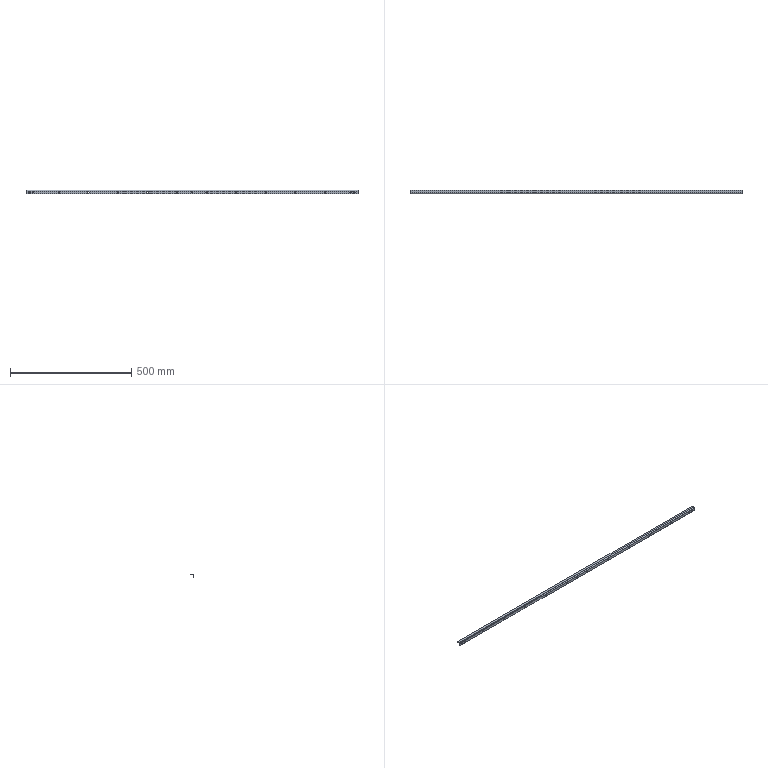Part | NX | features solid 2 | 1 solid | 40 faces | box 1368 x 13 x 15 mm | volume 66765 mm3 | cylinder 32 | plane 8 | commonest cylinder face diameters 6 x30 4 x1 8 x1
STEP:
#1=CARTESIAN_POINT('',(-726.,-675.5,1005.5));
#2=VERTEX_POINT('',#1);
#3=CARTESIAN_POINT('',(-726.,-677.5,1005.5));
#4=VERTEX_POINT('',#3);
#5=CARTESIAN_POINT('',(-726.,-2044.644,1005.5));
#6=DIRECTION('',(0.,1.,0.));
#7=VECTOR('',#6,1000.);
#8=LINE('',#5,#7);
#9=EDGE_CURVE('',#2,#4,#8,.F.);
#10=ORIENTED_EDGE('',*,*,#9,.T.);
#11=CARTESIAN_POINT('',(-726.,-677.5,999.5));
#12=VERTEX_POINT('',#11);
#13=CARTESIAN_POINT('',(-726.,-677.5,1002.5));
#14=DIRECTION('',(0.,-1.,0.));
#15=DIRECTION('',(1.,0.,0.));
#16=AXIS2_PLACEMENT_3D('',#13,#14,#15);
#17=CIRCLE('',#16,3.);
#18=EDGE_CURVE('',#4,#12,#17,.T.);
#19=ORIENTED_EDGE('',*,*,#18,.T.);
#20=CARTESIAN_POINT('',(-726.,-675.5,999.5));
#21=VERTEX_POINT('',#20);
#22=CARTESIAN_POINT('',(-726.,-2044.644,999.5));
#23=DIRECTION('',(0.,1.,0.));
#24=VECTOR('',#23,1000.);
#25=LINE('',#22,#24);
#26=EDGE_CURVE('',#12,#21,#25,.T.);
#27=ORIENTED_EDGE('',*,*,#26,.T.);
#28=CARTESIAN_POINT('',(-726.,-675.5,1002.5));
#29=DIRECTION('',(0.,1.,0.));
#30=DIRECTION('',(-1.,0.,0.));
#31=AXIS2_PLACEMENT_3D('',#28,#29,#30);
#32=CIRCLE('',#31,3.);
#33=EDGE_CURVE('',#21,#2,#32,.T.);
#34=ORIENTED_EDGE('',*,*,#33,.T.);
#35=EDGE_LOOP('',(#10,#19,#27,#34));
#36=FACE_BOUND('',#35,.T.);
#37=CARTESIAN_POINT('',(-726.,-2044.644,1002.5));
#38=DIRECTION('',(0.,1.,0.));
#39=DIRECTION('',(0.,0.,-1.));
#40=AXIS2_PLACEMENT_3D('',#37,#38,#39);
#41=CYLINDRICAL_SURFACE('',#40,3.);
#42=ADVANCED_FACE('',(#36),#41,.F.);
#43=CARTESIAN_POINT('',(-604.273,-677.5,1005.5));
#44=VERTEX_POINT('',#43);
#45=CARTESIAN_POINT('',(-604.273,-675.5,1005.5));
#46=VERTEX_POINT('',#45);
#47=CARTESIAN_POINT('',(-604.273,-2044.644,1005.5));
#48=DIRECTION('',(0.,1.,0.));
#49=VECTOR('',#48,1000.);
#50=LINE('',#47,#49);
#51=EDGE_CURVE('',#44,#46,#50,.T.);
#52=ORIENTED_EDGE('',*,*,#51,.F.);
#53=CARTESIAN_POINT('',(-604.273,-677.5,999.5));
#54=VERTEX_POINT('',#53);
#55=CARTESIAN_POINT('',(-604.273,-677.5,1002.5));
#56=DIRECTION('',(0.,-1.,0.));
#57=DIRECTION('',(1.,0.,0.));
#58=AXIS2_PLACEMENT_3D('',#55,#56,#57);
#59=CIRCLE('',#58,3.);
#60=EDGE_CURVE('',#44,#54,#59,.T.);
#61=ORIENTED_EDGE('',*,*,#60,.T.);
#62=CARTESIAN_POINT('',(-604.273,-675.5,999.5));
#63=VERTEX_POINT('',#62);
#64=CARTESIAN_POINT('',(-604.273,-2044.644,999.5));
#65=DIRECTION('',(0.,1.,0.));
#66=VECTOR('',#65,1000.);
#67=LINE('',#64,#66);
#68=EDGE_CURVE('',#63,#54,#67,.F.);
#69=ORIENTED_EDGE('',*,*,#68,.F.);
#70=CARTESIAN_POINT('',(-604.273,-675.5,1002.5));
#71=DIRECTION('',(0.,1.,0.));
#72=DIRECTION('',(-1.,0.,0.));
#73=AXIS2_PLACEMENT_3D('',#70,#71,#72);
#74=CIRCLE('',#73,3.);
#75=EDGE_CURVE('',#63,#46,#74,.T.);
#76=ORIENTED_EDGE('',*,*,#75,.T.);
#77=EDGE_LOOP('',(#52,#61,#69,#76));
#78=FACE_BOUND('',#77,.T.);
#79=CARTESIAN_POINT('',(-604.273,-2044.644,1002.5));
#80=DIRECTION('',(0.,1.,0.));
#81=DIRECTION('',(0.,0.,-1.));
#82=AXIS2_PLACEMENT_3D('',#79,#80,#81);
#83=CYLINDRICAL_SURFACE('',#82,3.);
#84=ADVANCED_FACE('',(#78),#83,.F.);
#85=CARTESIAN_POINT('',(-482.545,-675.5,1005.5));
#86=VERTEX_POINT('',#85);
#87=CARTESIAN_POINT('',(-482.545,-677.5,1005.5));
#88=VERTEX_POINT('',#87);
#89=CARTESIAN_POINT('',(-482.545,-2044.644,1005.5));
#90=DIRECTION('',(0.,1.,0.));
#91=VECTOR('',#90,1000.);
#92=LINE('',#89,#91);
#93=EDGE_CURVE('',#86,#88,#92,.F.);
#94=ORIENTED_EDGE('',*,*,#93,.T.);
#95=CARTESIAN_POINT('',(-482.545,-677.5,999.5));
#96=VERTEX_POINT('',#95);
#97=CARTESIAN_POINT('',(-482.545,-677.5,1002.5));
#98=DIRECTION('',(0.,-1.,0.));
#99=DIRECTION('',(1.,0.,0.));
#100=AXIS2_PLACEMENT_3D('',#97,#98,#99);
#101=CIRCLE('',#100,3.);
#102=EDGE_CURVE('',#88,#96,#101,.T.);
#103=ORIENTED_EDGE('',*,*,#102,.T.);
#104=CARTESIAN_POINT('',(-482.545,-675.5,999.5));
#105=VERTEX_POINT('',#104);
#106=CARTESIAN_POINT('',(-482.545,-2044.644,999.5));
#107=DIRECTION('',(0.,1.,0.));
#108=VECTOR('',#107,1000.);
#109=LINE('',#106,#108);
#110=EDGE_CURVE('',#96,#105,#109,.T.);
#111=ORIENTED_EDGE('',*,*,#110,.T.);
#112=CARTESIAN_POINT('',(-482.545,-675.5,1002.5));
#113=DIRECTION('',(0.,1.,0.));
#114=DIRECTION('',(-1.,0.,0.));
#115=AXIS2_PLACEMENT_3D('',#112,#113,#114);
#116=CIRCLE('',#115,3.);
#117=EDGE_CURVE('',#105,#86,#116,.T.);
#118=ORIENTED_EDGE('',*,*,#117,.T.);
#119=EDGE_LOOP('',(#94,#103,#111,#118));
#120=FACE_BOUND('',#119,.T.);
#121=CARTESIAN_POINT('',(-482.545,-2044.644,1002.5));
#122=DIRECTION('',(0.,1.,0.));
#123=DIRECTION('',(0.,0.,-1.));
#124=AXIS2_PLACEMENT_3D('',#121,#122,#123);
#125=CYLINDRICAL_SURFACE('',#124,3.);
#126=ADVANCED_FACE('',(#120),#125,.F.);
#127=CARTESIAN_POINT('',(-360.818,-675.5,1005.5));
#128=VERTEX_POINT('',#127);
#129=CARTESIAN_POINT('',(-360.818,-677.5,1005.5));
#130=VERTEX_POINT('',#129);
#131=CARTESIAN_POINT('',(-360.818,-2044.644,1005.5));
#132=DIRECTION('',(0.,1.,0.));
#133=VECTOR('',#132,1000.);
#134=LINE('',#131,#133);
#135=EDGE_CURVE('',#128,#130,#134,.F.);
#136=ORIENTED_EDGE('',*,*,#135,.T.);
#137=CARTESIAN_POINT('',(-360.818,-677.5,999.5));
#138=VERTEX_POINT('',#137);
#139=CARTESIAN_POINT('',(-360.818,-677.5,1002.5));
#140=DIRECTION('',(0.,-1.,0.));
#141=DIRECTION('',(1.,0.,0.));
#142=AXIS2_PLACEMENT_3D('',#139,#140,#141);
#143=CIRCLE('',#142,3.);
#144=EDGE_CURVE('',#130,#138,#143,.T.);
#145=ORIENTED_EDGE('',*,*,#144,.T.);
#146=CARTESIAN_POINT('',(-360.818,-675.5,999.5));
#147=VERTEX_POINT('',#146);
#148=CARTESIAN_POINT('',(-360.818,-2044.644,999.5));
#149=DIRECTION('',(0.,1.,0.));
#150=VECTOR('',#149,1000.);
#151=LINE('',#148,#150);
#152=EDGE_CURVE('',#138,#147,#151,.T.);
#153=ORIENTED_EDGE('',*,*,#152,.T.);
#154=CARTESIAN_POINT('',(-360.818,-675.5,1002.5));
#155=DIRECTION('',(0.,1.,0.));
#156=DIRECTION('',(-1.,0.,0.));
#157=AXIS2_PLACEMENT_3D('',#154,#155,#156);
#158=CIRCLE('',#157,3.);
#159=EDGE_CURVE('',#147,#128,#158,.T.);
#160=ORIENTED_EDGE('',*,*,#159,.T.);
#161=EDGE_LOOP('',(#136,#145,#153,#160));
#162=FACE_BOUND('',#161,.T.);
#163=CARTESIAN_POINT('',(-360.818,-2044.644,1002.5));
#164=DIRECTION('',(0.,1.,0.));
#165=DIRECTION('',(0.,0.,-1.));
#166=AXIS2_PLACEMENT_3D('',#163,#164,#165);
#167=CYLINDRICAL_SURFACE('',#166,3.);
#168=ADVANCED_FACE('',(#162),#167,.F.);
#169=CARTESIAN_POINT('',(-239.091,-677.5,1005.5));
#170=VERTEX_POINT('',#169);
#171=CARTESIAN_POINT('',(-239.091,-675.5,1005.5));
#172=VERTEX_POINT('',#171);
#173=CARTESIAN_POINT('',(-239.091,-2044.644,1005.5));
#174=DIRECTION('',(0.,1.,0.));
#175=VECTOR('',#174,1000.);
#176=LINE('',#173,#175);
#177=EDGE_CURVE('',#170,#172,#176,.T.);
#178=ORIENTED_EDGE('',*,*,#177,.F.);
#179=CARTESIAN_POINT('',(-239.091,-677.5,999.5));
#180=VERTEX_POINT('',#179);
#181=CARTESIAN_POINT('',(-239.091,-677.5,1002.5));
#182=DIRECTION('',(0.,-1.,0.));
#183=DIRECTION('',(1.,0.,0.));
#184=AXIS2_PLACEMENT_3D('',#181,#182,#183);
#185=CIRCLE('',#184,3.);
#186=EDGE_CURVE('',#170,#180,#185,.T.);
#187=ORIENTED_EDGE('',*,*,#186,.T.);
#188=CARTESIAN_POINT('',(-239.091,-675.5,999.5));
#189=VERTEX_POINT('',#188);
#190=CARTESIAN_POINT('',(-239.091,-2044.644,999.5));
#191=DIRECTION('',(0.,1.,0.));
#192=VECTOR('',#191,1000.);
#193=LINE('',#190,#192);
#194=EDGE_CURVE('',#189,#180,#193,.F.);
#195=ORIENTED_EDGE('',*,*,#194,.F.);
#196=CARTESIAN_POINT('',(-239.091,-675.5,1002.5));
#197=DIRECTION('',(0.,1.,0.));
#198=DIRECTION('',(-1.,0.,0.));
#199=AXIS2_PLACEMENT_3D('',#196,#197,#198);
#200=CIRCLE('',#199,3.);
#201=EDGE_CURVE('',#189,#172,#200,.T.);
#202=ORIENTED_EDGE('',*,*,#201,.T.);
#203=EDGE_LOOP('',(#178,#187,#195,#202));
#204=FACE_BOUND('',#203,.T.);
#205=CARTESIAN_POINT('',(-239.091,-2044.644,1002.5));
#206=DIRECTION('',(0.,1.,0.));
#207=DIRECTION('',(0.,0.,-1.));
#208=AXIS2_PLACEMENT_3D('',#205,#206,#207);
#209=CYLINDRICAL_SURFACE('',#208,3.);
#210=ADVANCED_FACE('',(#204),#209,.F.);
#211=CARTESIAN_POINT('',(-117.364,-675.5,1005.5));
#212=VERTEX_POINT('',#211);
#213=CARTESIAN_POINT('',(-117.364,-677.5,1005.5));
#214=VERTEX_POINT('',#213);
#215=CARTESIAN_POINT('',(-117.364,-2044.644,1005.5));
#216=DIRECTION('',(0.,1.,0.));
#217=VECTOR('',#216,1000.);
#218=LINE('',#215,#217);
#219=EDGE_CURVE('',#212,#214,#218,.F.);
#220=ORIENTED_EDGE('',*,*,#219,.T.);
#221=CARTESIAN_POINT('',(-117.364,-677.5,999.5));
#222=VERTEX_POINT('',#221);
#223=CARTESIAN_POINT('',(-117.364,-677.5,1002.5));
#224=DIRECTION('',(0.,-1.,0.));
#225=DIRECTION('',(1.,0.,0.));
#226=AXIS2_PLACEMENT_3D('',#223,#224,#225);
#227=CIRCLE('',#226,3.);
#228=EDGE_CURVE('',#214,#222,#227,.T.);
#229=ORIENTED_EDGE('',*,*,#228,.T.);
#230=CARTESIAN_POINT('',(-117.364,-675.5,999.5));
#231=VERTEX_POINT('',#230);
#232=CARTESIAN_POINT('',(-117.364,-2044.644,999.5));
#233=DIRECTION('',(0.,1.,0.));
#234=VECTOR('',#233,1000.);
#235=LINE('',#232,#234);
#236=EDGE_CURVE('',#222,#231,#235,.T.);
#237=ORIENTED_EDGE('',*,*,#236,.T.);
#238=CARTESIAN_POINT('',(-117.364,-675.5,1002.5));
#239=DIRECTION('',(0.,1.,0.));
#240=DIRECTION('',(-1.,0.,0.));
#241=AXIS2_PLACEMENT_3D('',#238,#239,#240);
#242=CIRCLE('',#241,3.);
#243=EDGE_CURVE('',#231,#212,#242,.T.);
#244=ORIENTED_EDGE('',*,*,#243,.T.);
#245=EDGE_LOOP('',(#220,#229,#237,#244));
#246=FACE_BOUND('',#245,.T.);
#247=CARTESIAN_POINT('',(-117.364,-2044.644,1002.5));
#248=DIRECTION('',(0.,1.,0.));
#249=DIRECTION('',(0.,0.,-1.));
#250=AXIS2_PLACEMENT_3D('',#247,#248,#249);
#251=CYLINDRICAL_SURFACE('',#250,3.);
#252=ADVANCED_FACE('',(#246),#251,.F.);
#253=CARTESIAN_POINT('',(4.364,-677.5,1005.5));
#254=VERTEX_POINT('',#253);
#255=CARTESIAN_POINT('',(4.364,-675.5,1005.5));
#256=VERTEX_POINT('',#255);
#257=CARTESIAN_POINT('',(4.364,-2044.644,1005.5));
#258=DIRECTION('',(0.,1.,0.));
#259=VECTOR('',#258,1000.);
#260=LINE('',#257,#259);
#261=EDGE_CURVE('',#254,#256,#260,.T.);
#262=ORIENTED_EDGE('',*,*,#261,.F.);
#263=CARTESIAN_POINT('',(4.364,-677.5,999.5));
#264=VERTEX_POINT('',#263);
#265=CARTESIAN_POINT('',(4.364,-677.5,1002.5));
#266=DIRECTION('',(0.,-1.,0.));
#267=DIRECTION('',(1.,0.,0.));
#268=AXIS2_PLACEMENT_3D('',#265,#266,#267);
#269=CIRCLE('',#268,3.);
#270=EDGE_CURVE('',#254,#264,#269,.T.);
#271=ORIENTED_EDGE('',*,*,#270,.T.);
#272=CARTESIAN_POINT('',(4.364,-675.5,999.5));
#273=VERTEX_POINT('',#272);
#274=CARTESIAN_POINT('',(4.364,-2044.644,999.5));
#275=DIRECTION('',(0.,1.,0.));
#276=VECTOR('',#275,1000.);
#277=LINE('',#274,#276);
#278=EDGE_CURVE('',#273,#264,#277,.F.);
#279=ORIENTED_EDGE('',*,*,#278,.F.);
#280=CARTESIAN_POINT('',(4.364,-675.5,1002.5));
#281=DIRECTION('',(0.,1.,0.));
#282=DIRECTION('',(-1.,0.,0.));
#283=AXIS2_PLACEMENT_3D('',#280,#281,#282);
#284=CIRCLE('',#283,3.);
#285=EDGE_CURVE('',#273,#256,#284,.T.);
#286=ORIENTED_EDGE('',*,*,#285,.T.);
#287=EDGE_LOOP('',(#262,#271,#279,#286));
#288=FACE_BOUND('',#287,.T.);
#289=CARTESIAN_POINT('',(4.364,-2044.644,1002.5));
#290=DIRECTION('',(0.,1.,0.));
#291=DIRECTION('',(0.,0.,-1.));
#292=AXIS2_PLACEMENT_3D('',#289,#290,#291);
#293=CYLINDRICAL_SURFACE('',#292,3.);
#294=ADVANCED_FACE('',(#288),#293,.F.);
#295=CARTESIAN_POINT('',(126.091,-675.5,1005.5));
#296=VERTEX_POINT('',#295);
#297=CARTESIAN_POINT('',(126.091,-677.5,1005.5));
#298=VERTEX_POINT('',#297);
#299=CARTESIAN_POINT('',(126.091,-2044.644,1005.5));
#300=DIRECTION('',(0.,1.,0.));
#301=VECTOR('',#300,1000.);
#302=LINE('',#299,#301);
#303=EDGE_CURVE('',#296,#298,#302,.F.);
#304=ORIENTED_EDGE('',*,*,#303,.T.);
#305=CARTESIAN_POINT('',(126.091,-677.5,999.5));
#306=VERTEX_POINT('',#305);
#307=CARTESIAN_POINT('',(126.091,-677.5,1002.5));
#308=DIRECTION('',(0.,-1.,0.));
#309=DIRECTION('',(1.,0.,0.));
#310=AXIS2_PLACEMENT_3D('',#307,#308,#309);
#311=CIRCLE('',#310,3.);
#312=EDGE_CURVE('',#298,#306,#311,.T.);
#313=ORIENTED_EDGE('',*,*,#312,.T.);
#314=CARTESIAN_POINT('',(126.091,-675.5,999.5));
#315=VERTEX_POINT('',#314);
#316=CARTESIAN_POINT('',(126.091,-2044.644,999.5));
#317=DIRECTION('',(0.,1.,0.));
#318=VECTOR('',#317,1000.);
#319=LINE('',#316,#318);
#320=EDGE_CURVE('',#306,#315,#319,.T.);
#321=ORIENTED_EDGE('',*,*,#320,.T.);
#322=CARTESIAN_POINT('',(126.091,-675.5,1002.5));
#323=DIRECTION('',(0.,1.,0.));
#324=DIRECTION('',(-1.,0.,0.));
#325=AXIS2_PLACEMENT_3D('',#322,#323,#324);
#326=CIRCLE('',#325,3.);
#327=EDGE_CURVE('',#315,#296,#326,.T.);
#328=ORIENTED_EDGE('',*,*,#327,.T.);
#329=EDGE_LOOP('',(#304,#313,#321,#328));
#330=FACE_BOUND('',#329,.T.);
#331=CARTESIAN_POINT('',(126.091,-2044.644,1002.5));
#332=DIRECTION('',(0.,1.,0.));
#333=DIRECTION('',(0.,0.,-1.));
#334=AXIS2_PLACEMENT_3D('',#331,#332,#333);
#335=CYLINDRICAL_SURFACE('',#334,3.);
#336=ADVANCED_FACE('',(#330),#335,.F.);
#337=CARTESIAN_POINT('',(247.818,-675.5,1005.5));
#338=VERTEX_POINT('',#337);
#339=CARTESIAN_POINT('',(247.818,-677.5,1005.5));
#340=VERTEX_POINT('',#339);
#341=CARTESIAN_POINT('',(247.818,-2044.644,1005.5));
#342=DIRECTION('',(0.,1.,0.));
#343=VECTOR('',#342,1000.);
#344=LINE('',#341,#343);
#345=EDGE_CURVE('',#338,#340,#344,.F.);
#346=ORIENTED_EDGE('',*,*,#345,.T.);
#347=CARTESIAN_POINT('',(247.818,-677.5,999.5));
#348=VERTEX_POINT('',#347);
#349=CARTESIAN_POINT('',(247.818,-677.5,1002.5));
#350=DIRECTION('',(0.,-1.,0.));
#351=DIRECTION('',(1.,0.,0.));
#352=AXIS2_PLACEMENT_3D('',#349,#350,#351);
#353=CIRCLE('',#352,3.);
#354=EDGE_CURVE('',#340,#348,#353,.T.);
#355=ORIENTED_EDGE('',*,*,#354,.T.);
#356=CARTESIAN_POINT('',(247.818,-675.5,999.5));
#357=VERTEX_POINT('',#356);
#358=CARTESIAN_POINT('',(247.818,-2044.644,999.5));
#359=DIRECTION('',(0.,1.,0.));
#360=VECTOR('',#359,1000.);
#361=LINE('',#358,#360);
#362=EDGE_CURVE('',#348,#357,#361,.T.);
#363=ORIENTED_EDGE('',*,*,#362,.T.);
#364=CARTESIAN_POINT('',(247.818,-675.5,1002.5));
#365=DIRECTION('',(0.,1.,0.));
#366=DIRECTION('',(-1.,0.,0.));
#367=AXIS2_PLACEMENT_3D('',#364,#365,#366);
#368=CIRCLE('',#367,3.);
#369=EDGE_CURVE('',#357,#338,#368,.T.);
#370=ORIENTED_EDGE('',*,*,#369,.T.);
#371=EDGE_LOOP('',(#346,#355,#363,#370));
#372=FACE_BOUND('',#371,.T.);
#373=CARTESIAN_POINT('',(247.818,-2044.644,1002.5));
#374=DIRECTION('',(0.,1.,0.));
#375=DIRECTION('',(0.,0.,-1.));
#376=AXIS2_PLACEMENT_3D('',#373,#374,#375);
#377=CYLINDRICAL_SURFACE('',#376,3.);
#378=ADVANCED_FACE('',(#372),#377,.F.);
#379=CARTESIAN_POINT('',(369.545,-677.5,1005.5));
#380=VERTEX_POINT('',#379);
#381=CARTESIAN_POINT('',(369.545,-675.5,1005.5));
#382=VERTEX_POINT('',#381);
#383=CARTESIAN_POINT('',(369.545,-2044.644,1005.5));
#384=DIRECTION('',(0.,1.,0.));
#385=VECTOR('',#384,1000.);
#386=LINE('',#383,#385);
#387=EDGE_CURVE('',#380,#382,#386,.T.);
#388=ORIENTED_EDGE('',*,*,#387,.F.);
#389=CARTESIAN_POINT('',(369.545,-677.5,999.5));
#390=VERTEX_POINT('',#389);
#391=CARTESIAN_POINT('',(369.545,-677.5,1002.5));
#392=DIRECTION('',(0.,-1.,0.));
#393=DIRECTION('',(1.,0.,0.));
#394=AXIS2_PLACEMENT_3D('',#391,#392,#393);
#395=CIRCLE('',#394,3.);
#396=EDGE_CURVE('',#380,#390,#395,.T.);
#397=ORIENTED_EDGE('',*,*,#396,.T.);
#398=CARTESIAN_POINT('',(369.545,-675.5,999.5));
#399=VERTEX_POINT('',#398);
#400=CARTESIAN_POINT('',(369.545,-2044.644,999.5));
#401=DIRECTION('',(0.,1.,0.));
#402=VECTOR('',#401,1000.);
#403=LINE('',#400,#402);
#404=EDGE_CURVE('',#399,#390,#403,.F.);
#405=ORIENTED_EDGE('',*,*,#404,.F.);
#406=CARTESIAN_POINT('',(369.545,-675.5,1002.5));
#407=DIRECTION('',(0.,1.,0.));
#408=DIRECTION('',(-1.,0.,0.));
#409=AXIS2_PLACEMENT_3D('',#406,#407,#408);
#410=CIRCLE('',#409,3.);
#411=EDGE_CURVE('',#399,#382,#410,.T.);
#412=ORIENTED_EDGE('',*,*,#411,.T.);
#413=EDGE_LOOP('',(#388,#397,#405,#412));
#414=FACE_BOUND('',#413,.T.);
#415=CARTESIAN_POINT('',(369.545,-2044.644,1002.5));
#416=DIRECTION('',(0.,1.,0.));
#417=DIRECTION('',(0.,0.,-1.));
#418=AXIS2_PLACEMENT_3D('',#415,#416,#417);
#419=CYLINDRICAL_SURFACE('',#418,3.);
#420=ADVANCED_FACE('',(#414),#419,.F.);
#421=CARTESIAN_POINT('',(491.273,-675.5,1005.5));
#422=VERTEX_POINT('',#421);
#423=CARTESIAN_POINT('',(491.273,-677.5,1005.5));
#424=VERTEX_POINT('',#423);
#425=CARTESIAN_POINT('',(491.273,-2044.644,1005.5));
#426=DIRECTION('',(0.,1.,0.));
#427=VECTOR('',#426,1000.);
#428=LINE('',#425,#427);
#429=EDGE_CURVE('',#422,#424,#428,.F.);
#430=ORIENTED_EDGE('',*,*,#429,.T.);
#431=CARTESIAN_POINT('',(491.273,-677.5,999.5));
#432=VERTEX_POINT('',#431);
#433=CARTESIAN_POINT('',(491.273,-677.5,1002.5));
#434=DIRECTION('',(0.,-1.,0.));
#435=DIRECTION('',(1.,0.,0.));
#436=AXIS2_PLACEMENT_3D('',#433,#434,#435);
#437=CIRCLE('',#436,3.);
#438=EDGE_CURVE('',#424,#432,#437,.T.);
#439=ORIENTED_EDGE('',*,*,#438,.T.);
#440=CARTESIAN_POINT('',(491.273,-675.5,999.5));
#441=VERTEX_POINT('',#440);
#442=CARTESIAN_POINT('',(491.273,-2044.644,999.5));
#443=DIRECTION('',(0.,1.,0.));
#444=VECTOR('',#443,1000.);
#445=LINE('',#442,#444);
#446=EDGE_CURVE('',#432,#441,#445,.T.);
#447=ORIENTED_EDGE('',*,*,#446,.T.);
#448=CARTESIAN_POINT('',(491.273,-675.5,1002.5));
#449=DIRECTION('',(0.,1.,0.));
#450=DIRECTION('',(-1.,0.,0.));
#451=AXIS2_PLACEMENT_3D('',#448,#449,#450);
#452=CIRCLE('',#451,3.);
#453=EDGE_CURVE('',#441,#422,#452,.T.);
#454=ORIENTED_EDGE('',*,*,#453,.T.);
#455=EDGE_LOOP('',(#430,#439,#447,#454));
#456=FACE_BOUND('',#455,.T.);
#457=CARTESIAN_POINT('',(491.273,-2044.644,1002.5));
#458=DIRECTION('',(0.,1.,0.));
#459=DIRECTION('',(0.,0.,-1.));
#460=AXIS2_PLACEMENT_3D('',#457,#458,#459);
#461=CYLINDRICAL_SURFACE('',#460,3.);
#462=ADVANCED_FACE('',(#456),#461,.F.);
#463=CARTESIAN_POINT('',(613.,-675.5,1005.5));
#464=VERTEX_POINT('',#463);
#465=CARTESIAN_POINT('',(613.,-677.5,1005.5));
#466=VERTEX_POINT('',#465);
#467=CARTESIAN_POINT('',(613.,-2044.644,1005.5));
#468=DIRECTION('',(0.,1.,0.));
#469=VECTOR('',#468,1000.);
#470=LINE('',#467,#469);
#471=EDGE_CURVE('',#464,#466,#470,.F.);
#472=ORIENTED_EDGE('',*,*,#471,.T.);
#473=CARTESIAN_POINT('',(613.,-677.5,999.5));
#474=VERTEX_POINT('',#473);
#475=CARTESIAN_POINT('',(613.,-677.5,1002.5));
#476=DIRECTION('',(0.,-1.,0.));
#477=DIRECTION('',(1.,0.,0.));
#478=AXIS2_PLACEMENT_3D('',#475,#476,#477);
#479=CIRCLE('',#478,3.);
#480=EDGE_CURVE('',#466,#474,#479,.T.);
#481=ORIENTED_EDGE('',*,*,#480,.T.);
#482=CARTESIAN_POINT('',(613.,-675.5,999.5));
#483=VERTEX_POINT('',#482);
#484=CARTESIAN_POINT('',(613.,-2044.644,999.5));
#485=DIRECTION('',(0.,1.,0.));
#486=VECTOR('',#485,1000.);
#487=LINE('',#484,#486);
#488=EDGE_CURVE('',#474,#483,#487,.T.);
#489=ORIENTED_EDGE('',*,*,#488,.T.);
#490=CARTESIAN_POINT('',(613.,-675.5,1002.5));
#491=DIRECTION('',(0.,1.,0.));
#492=DIRECTION('',(-1.,0.,0.));
#493=AXIS2_PLACEMENT_3D('',#490,#491,#492);
#494=CIRCLE('',#493,3.);
#495=EDGE_CURVE('',#483,#464,#494,.T.);
#496=ORIENTED_EDGE('',*,*,#495,.T.);
#497=EDGE_LOOP('',(#472,#481,#489,#496));
#498=FACE_BOUND('',#497,.T.);
#499=CARTESIAN_POINT('',(613.,-2044.644,1002.5));
#500=DIRECTION('',(0.,1.,0.));
#501=DIRECTION('',(0.,0.,-1.));
#502=AXIS2_PLACEMENT_3D('',#499,#500,#501);
#503=CYLINDRICAL_SURFACE('',#502,3.);
#504=ADVANCED_FACE('',(#498),#503,.F.);
#505=CARTESIAN_POINT('',(-740.,-664.5,1010.));
#506=VERTEX_POINT('',#505);
#507=CARTESIAN_POINT('',(-740.,-673.5,1010.));
#508=VERTEX_POINT('',#507);
#509=CARTESIAN_POINT('',(-740.,-677.5,1010.));
#510=DIRECTION('',(0.,-1.,0.));
#511=VECTOR('',#510,1000.);
#512=LINE('',#509,#511);
#513=EDGE_CURVE('',#506,#508,#512,.T.);
#514=ORIENTED_EDGE('',*,*,#513,.T.);
#515=CARTESIAN_POINT('',(-740.,-675.5,1008.));
#516=VERTEX_POINT('',#515);
#517=CARTESIAN_POINT('',(-740.,-673.5,1008.));
#518=DIRECTION('',(1.,0.,0.));
#519=DIRECTION('',(0.,1.,0.));
#520=AXIS2_PLACEMENT_3D('',#517,#518,#519);
#521=CIRCLE('',#520,2.);
#522=EDGE_CURVE('',#508,#516,#521,.T.);
#523=ORIENTED_EDGE('',*,*,#522,.T.);
#524=CARTESIAN_POINT('',(-740.,-675.5,997.));
#525=VERTEX_POINT('',#524);
#526=CARTESIAN_POINT('',(-740.,-675.5,1012.));
#527=DIRECTION('',(0.,0.,-1.));
#528=VECTOR('',#527,1000.);
#529=LINE('',#526,#528);
#530=EDGE_CURVE('',#516,#525,#529,.T.);
#531=ORIENTED_EDGE('',*,*,#530,.T.);
#532=CARTESIAN_POINT('',(-740.,-677.5,997.));
#533=VERTEX_POINT('',#532);
#534=CARTESIAN_POINT('',(-740.,-677.5,997.));
#535=DIRECTION('',(0.,1.,0.));
#536=VECTOR('',#535,1000.);
#537=LINE('',#534,#536);
#538=EDGE_CURVE('',#533,#525,#537,.T.);
#539=ORIENTED_EDGE('',*,*,#538,.F.);
#540=CARTESIAN_POINT('',(-740.,-677.5,1008.));
#541=VERTEX_POINT('',#540);
#542=CARTESIAN_POINT('',(-740.,-677.5,1012.));
#543=DIRECTION('',(0.,0.,-1.));
#544=VECTOR('',#543,1000.);
#545=LINE('',#542,#544);
#546=EDGE_CURVE('',#541,#533,#545,.T.);
#547=ORIENTED_EDGE('',*,*,#546,.F.);
#548=CARTESIAN_POINT('',(-740.,-673.5,1012.));
#549=VERTEX_POINT('',#548);
#550=CARTESIAN_POINT('',(-740.,-673.5,1008.));
#551=DIRECTION('',(1.,0.,0.));
#552=DIRECTION('',(0.,-1.,0.));
#553=AXIS2_PLACEMENT_3D('',#550,#551,#552);
#554=CIRCLE('',#553,4.);
#555=EDGE_CURVE('',#549,#541,#554,.T.);
#556=ORIENTED_EDGE('',*,*,#555,.F.);
#557=CARTESIAN_POINT('',(-740.,-664.5,1012.));
#558=VERTEX_POINT('',#557);
#559=CARTESIAN_POINT('',(-740.,-677.5,1012.));
#560=DIRECTION('',(0.,-1.,0.));
#561=VECTOR('',#560,1000.);
#562=LINE('',#559,#561);
#563=EDGE_CURVE('',#558,#549,#562,.T.);
#564=ORIENTED_EDGE('',*,*,#563,.F.);
#565=CARTESIAN_POINT('',(-740.,-664.5,1010.));
#566=DIRECTION('',(0.,0.,1.));
#567=VECTOR('',#566,1000.);
#568=LINE('',#565,#567);
#569=EDGE_CURVE('',#506,#558,#568,.T.);
#570=ORIENTED_EDGE('',*,*,#569,.F.);
#571=EDGE_LOOP('',(#514,#523,#531,#539,#547,#556,#564,#570));
#572=FACE_BOUND('',#571,.T.);
#573=CARTESIAN_POINT('',(-740.,-677.5,1009.5));
#574=DIRECTION('',(-1.,0.,0.));
#575=DIRECTION('',(0.,1.,0.));
#576=AXIS2_PLACEMENT_3D('',#573,#574,#575);
#577=PLANE('',#576);
#578=ADVANCED_FACE('',(#572),#577,.T.);
#579=CARTESIAN_POINT('',(628.,-664.5,1012.));
#580=VERTEX_POINT('',#579);
#581=CARTESIAN_POINT('',(628.,-673.5,1012.));
#582=VERTEX_POINT('',#581);
#583=CARTESIAN_POINT('',(628.,-677.5,1012.));
#584=DIRECTION('',(0.,-1.,0.));
#585=VECTOR('',#584,1000.);
#586=LINE('',#583,#585);
#587=EDGE_CURVE('',#580,#582,#586,.T.);
#588=ORIENTED_EDGE('',*,*,#587,.F.);
#589=CARTESIAN_POINT('',(-741.,-664.5,1012.));
#590=DIRECTION('',(1.,0.,0.));
#591=VECTOR('',#590,1000.);
#592=LINE('',#589,#591);
#593=EDGE_CURVE('',#558,#580,#592,.T.);
#594=ORIENTED_EDGE('',*,*,#593,.F.);
#595=ORIENTED_EDGE('',*,*,#563,.T.);
#596=CARTESIAN_POINT('',(-741.,-673.5,1012.));
#597=DIRECTION('',(1.,0.,0.));
#598=VECTOR('',#597,1000.);
#599=LINE('',#596,#598);
#600=EDGE_CURVE('',#549,#582,#599,.T.);
#601=ORIENTED_EDGE('',*,*,#600,.T.);
#602=EDGE_LOOP('',(#588,#594,#595,#601));
#603=FACE_BOUND('',#602,.T.);
#604=CARTESIAN_POINT('',(-741.,-677.5,1012.));
#605=DIRECTION('',(0.,0.,1.));
#606=DIRECTION('',(1.,0.,0.));
#607=AXIS2_PLACEMENT_3D('',#604,#605,#606);
#608=PLANE('',#607);
#609=ADVANCED_FACE('',(#603),#608,.T.);
#610=CARTESIAN_POINT('',(628.,-664.5,1010.));
#611=VERTEX_POINT('',#610);
#612=CARTESIAN_POINT('',(628.,-673.5,1010.));
#613=VERTEX_POINT('',#612);
#614=CARTESIAN_POINT('',(628.,-677.5,1010.));
#615=DIRECTION('',(0.,-1.,0.));
#616=VECTOR('',#615,1000.);
#617=LINE('',#614,#616);
#618=EDGE_CURVE('',#611,#613,#617,.T.);
#619=ORIENTED_EDGE('',*,*,#618,.T.);
#620=CARTESIAN_POINT('',(-741.,-673.5,1010.));
#621=DIRECTION('',(1.,0.,0.));
#622=VECTOR('',#621,1000.);
#623=LINE('',#620,#622);
#624=EDGE_CURVE('',#508,#613,#623,.T.);
#625=ORIENTED_EDGE('',*,*,#624,.F.);
#626=ORIENTED_EDGE('',*,*,#513,.F.);
#627=CARTESIAN_POINT('',(-741.,-664.5,1010.));
#628=DIRECTION('',(1.,0.,0.));
#629=VECTOR('',#628,1000.);
#630=LINE('',#627,#629);
#631=EDGE_CURVE('',#506,#611,#630,.T.);
#632=ORIENTED_EDGE('',*,*,#631,.T.);
#633=EDGE_LOOP('',(#619,#625,#626,#632));
#634=FACE_BOUND('',#633,.T.);
#635=CARTESIAN_POINT('',(-741.,-677.5,1010.));
#636=DIRECTION('',(0.,0.,1.));
#637=DIRECTION('',(1.,0.,0.));
#638=AXIS2_PLACEMENT_3D('',#635,#636,#637);
#639=PLANE('',#638);
#640=ADVANCED_FACE('',(#634),#639,.F.);
#641=CARTESIAN_POINT('',(628.,-664.5,1010.));
#642=DIRECTION('',(0.,0.,1.));
#643=VECTOR('',#642,1000.);
#644=LINE('',#641,#643);
#645=EDGE_CURVE('',#611,#580,#644,.T.);
#646=ORIENTED_EDGE('',*,*,#645,.F.);
#647=ORIENTED_EDGE('',*,*,#631,.F.);
#648=ORIENTED_EDGE('',*,*,#569,.T.);
#649=ORIENTED_EDGE('',*,*,#593,.T.);
#650=EDGE_LOOP('',(#646,#647,#648,#649));
#651=FACE_BOUND('',#650,.T.);
#652=CARTESIAN_POINT('',(-741.,-664.5,1010.));
#653=DIRECTION('',(0.,1.,0.));
#654=DIRECTION('',(0.,0.,-1.));
#655=AXIS2_PLACEMENT_3D('',#652,#653,#654);
#656=PLANE('',#655);
#657=ADVANCED_FACE('',(#651),#656,.T.);
#658=ORIENTED_EDGE('',*,*,#522,.F.);
#659=ORIENTED_EDGE('',*,*,#624,.T.);
#660=CARTESIAN_POINT('',(628.,-675.5,1008.));
#661=VERTEX_POINT('',#660);
#662=CARTESIAN_POINT('',(628.,-673.5,1008.));
#663=DIRECTION('',(1.,0.,0.));
#664=DIRECTION('',(0.,1.,0.));
#665=AXIS2_PLACEMENT_3D('',#662,#663,#664);
#666=CIRCLE('',#665,2.);
#667=EDGE_CURVE('',#613,#661,#666,.T.);
#668=ORIENTED_EDGE('',*,*,#667,.T.);
#669=CARTESIAN_POINT('',(-741.,-675.5,1008.));
#670=DIRECTION('',(1.,0.,0.));
#671=VECTOR('',#670,1000.);
#672=LINE('',#669,#671);
#673=EDGE_CURVE('',#516,#661,#672,.T.);
#674=ORIENTED_EDGE('',*,*,#673,.F.);
#675=EDGE_LOOP('',(#658,#659,#668,#674));
#676=FACE_BOUND('',#675,.T.);
#677=CARTESIAN_POINT('',(-741.,-673.5,1008.));
#678=DIRECTION('',(1.,0.,0.));
#679=DIRECTION('',(0.,-1.,0.));
#680=AXIS2_PLACEMENT_3D('',#677,#678,#679);
#681=CYLINDRICAL_SURFACE('',#680,2.);
#682=ADVANCED_FACE('',(#676),#681,.F.);
#683=ORIENTED_EDGE('',*,*,#555,.T.);
#684=CARTESIAN_POINT('',(628.,-677.5,1008.));
#685=VERTEX_POINT('',#684);
#686=CARTESIAN_POINT('',(-741.,-677.5,1008.));
#687=DIRECTION('',(1.,0.,0.));
#688=VECTOR('',#687,1000.);
#689=LINE('',#686,#688);
#690=EDGE_CURVE('',#541,#685,#689,.T.);
#691=ORIENTED_EDGE('',*,*,#690,.T.);
#692=CARTESIAN_POINT('',(628.,-673.5,1008.));
#693=DIRECTION('',(1.,0.,0.));
#694=DIRECTION('',(0.,-1.,0.));
#695=AXIS2_PLACEMENT_3D('',#692,#693,#694);
#696=CIRCLE('',#695,4.);
#697=EDGE_CURVE('',#582,#685,#696,.T.);
#698=ORIENTED_EDGE('',*,*,#697,.F.);
#699=ORIENTED_EDGE('',*,*,#600,.F.);
#700=EDGE_LOOP('',(#683,#691,#698,#699));
#701=FACE_BOUND('',#700,.T.);
#702=CARTESIAN_POINT('',(-741.,-673.5,1008.));
#703=DIRECTION('',(1.,0.,0.));
#704=DIRECTION('',(0.,-1.,0.));
#705=AXIS2_PLACEMENT_3D('',#702,#703,#704);
#706=CYLINDRICAL_SURFACE('',#705,4.);
#707=ADVANCED_FACE('',(#701),#706,.T.);
#708=CARTESIAN_POINT('',(-711.,-675.5,1007.));
#709=VERTEX_POINT('',#708);
#710=CARTESIAN_POINT('',(-711.,-677.5,1007.));
#711=VERTEX_POINT('',#710);
#712=CARTESIAN_POINT('',(-711.,-2012.147,1007.));
#713=DIRECTION('',(0.,1.,0.));
#714=VECTOR('',#713,1000.);
#715=LINE('',#712,#714);
#716=EDGE_CURVE('',#709,#711,#715,.F.);
#717=ORIENTED_EDGE('',*,*,#716,.T.);
#718=CARTESIAN_POINT('',(-711.,-677.5,1001.));
#719=VERTEX_POINT('',#718);
#720=CARTESIAN_POINT('',(-711.,-677.5,1004.));
#721=DIRECTION('',(0.,-1.,0.));
#722=DIRECTION('',(1.,0.,0.));
#723=AXIS2_PLACEMENT_3D('',#720,#721,#722);
#724=CIRCLE('',#723,3.);
#725=EDGE_CURVE('',#711,#719,#724,.T.);
#726=ORIENTED_EDGE('',*,*,#725,.T.);
#727=CARTESIAN_POINT('',(-711.,-675.5,1001.));
#728=VERTEX_POINT('',#727);
#729=CARTESIAN_POINT('',(-711.,-2012.147,1001.));
#730=DIRECTION('',(0.,1.,0.));
#731=VECTOR('',#730,1000.);
#732=LINE('',#729,#731);
#733=EDGE_CURVE('',#719,#728,#732,.T.);
#734=ORIENTED_EDGE('',*,*,#733,.T.);
#735=CARTESIAN_POINT('',(-711.,-675.5,1004.));
#736=DIRECTION('',(0.,1.,0.));
#737=DIRECTION('',(1.,0.,0.));
#738=AXIS2_PLACEMENT_3D('',#735,#736,#737);
#739=CIRCLE('',#738,3.);
#740=EDGE_CURVE('',#728,#709,#739,.T.);
#741=ORIENTED_EDGE('',*,*,#740,.T.);
#742=EDGE_LOOP('',(#717,#726,#734,#741));
#743=FACE_BOUND('',#742,.T.);
#744=CARTESIAN_POINT('',(-711.,-2012.147,1004.));
#745=DIRECTION('',(0.,1.,0.));
#746=DIRECTION('',(0.,0.,-1.));
#747=AXIS2_PLACEMENT_3D('',#744,#745,#746);
#748=CYLINDRICAL_SURFACE('',#747,3.);
#749=ADVANCED_FACE('',(#743),#748,.F.);
#750=CARTESIAN_POINT('',(-56.5,-677.5,1007.));
#751=VERTEX_POINT('',#750);
#752=CARTESIAN_POINT('',(-56.5,-675.5,1007.));
#753=VERTEX_POINT('',#752);
#754=CARTESIAN_POINT('',(-56.5,-2012.147,1007.));
#755=DIRECTION('',(0.,1.,0.));
#756=VECTOR('',#755,1000.);
#757=LINE('',#754,#756);
#758=EDGE_CURVE('',#751,#753,#757,.T.);
#759=ORIENTED_EDGE('',*,*,#758,.F.);
#760=CARTESIAN_POINT('',(-56.5,-677.5,1001.));
#761=VERTEX_POINT('',#760);
#762=CARTESIAN_POINT('',(-56.5,-677.5,1004.));
#763=DIRECTION('',(0.,-1.,0.));
#764=DIRECTION('',(1.,0.,0.));
#765=AXIS2_PLACEMENT_3D('',#762,#763,#764);
#766=CIRCLE('',#765,3.);
#767=EDGE_CURVE('',#751,#761,#766,.T.);
#768=ORIENTED_EDGE('',*,*,#767,.T.);
#769=CARTESIAN_POINT('',(-56.5,-675.5,1001.));
#770=VERTEX_POINT('',#769);
#771=CARTESIAN_POINT('',(-56.5,-2012.147,1001.));
#772=DIRECTION('',(0.,1.,0.));
#773=VECTOR('',#772,1000.);
#774=LINE('',#771,#773);
#775=EDGE_CURVE('',#770,#761,#774,.F.);
#776=ORIENTED_EDGE('',*,*,#775,.F.);
#777=CARTESIAN_POINT('',(-56.5,-675.5,1004.));
#778=DIRECTION('',(0.,1.,0.));
#779=DIRECTION('',(1.,0.,0.));
#780=AXIS2_PLACEMENT_3D('',#777,#778,#779);
#781=CIRCLE('',#780,3.);
#782=EDGE_CURVE('',#770,#753,#781,.T.);
#783=ORIENTED_EDGE('',*,*,#782,.T.);
#784=EDGE_LOOP('',(#759,#768,#776,#783));
#785=FACE_BOUND('',#784,.T.);
#786=CARTESIAN_POINT('',(-56.5,-2012.147,1004.));
#787=DIRECTION('',(0.,1.,0.));
#788=DIRECTION('',(0.,0.,-1.));
#789=AXIS2_PLACEMENT_3D('',#786,#787,#788);
#790=CYLINDRICAL_SURFACE('',#789,3.);
#791=ADVANCED_FACE('',(#785),#790,.F.);
#792=CARTESIAN_POINT('',(598.,-677.5,1007.));
#793=VERTEX_POINT('',#792);
#794=CARTESIAN_POINT('',(598.,-675.5,1007.));
#795=VERTEX_POINT('',#794);
#796=CARTESIAN_POINT('',(598.,-2012.147,1007.));
#797=DIRECTION('',(0.,1.,0.));
#798=VECTOR('',#797,1000.);
#799=LINE('',#796,#798);
#800=EDGE_CURVE('',#793,#795,#799,.T.);
#801=ORIENTED_EDGE('',*,*,#800,.F.);
#802=CARTESIAN_POINT('',(598.,-677.5,1001.));
#803=VERTEX_POINT('',#802);
#804=CARTESIAN_POINT('',(598.,-677.5,1004.));
#805=DIRECTION('',(0.,-1.,0.));
#806=DIRECTION('',(1.,0.,0.));
#807=AXIS2_PLACEMENT_3D('',#804,#805,#806);
#808=CIRCLE('',#807,3.);
#809=EDGE_CURVE('',#793,#803,#808,.T.);
#810=ORIENTED_EDGE('',*,*,#809,.T.);
#811=CARTESIAN_POINT('',(598.,-675.5,1001.));
#812=VERTEX_POINT('',#811);
#813=CARTESIAN_POINT('',(598.,-2012.147,1001.));
#814=DIRECTION('',(0.,1.,0.));
#815=VECTOR('',#814,1000.);
#816=LINE('',#813,#815);
#817=EDGE_CURVE('',#812,#803,#816,.F.);
#818=ORIENTED_EDGE('',*,*,#817,.F.);
#819=CARTESIAN_POINT('',(598.,-675.5,1004.));
#820=DIRECTION('',(0.,1.,0.));
#821=DIRECTION('',(1.,0.,0.));
#822=AXIS2_PLACEMENT_3D('',#819,#820,#821);
#823=CIRCLE('',#822,3.);
#824=EDGE_CURVE('',#812,#795,#823,.T.);
#825=ORIENTED_EDGE('',*,*,#824,.T.);
#826=EDGE_LOOP('',(#801,#810,#818,#825));
#827=FACE_BOUND('',#826,.T.);
#828=CARTESIAN_POINT('',(598.,-2012.147,1004.));
#829=DIRECTION('',(0.,1.,0.));
#830=DIRECTION('',(0.,0.,-1.));
#831=AXIS2_PLACEMENT_3D('',#828,#829,#830);
#832=CYLINDRICAL_SURFACE('',#831,3.);
#833=ADVANCED_FACE('',(#827),#832,.F.);
#834=ORIENTED_EDGE('',*,*,#824,.F.);
#835=CARTESIAN_POINT('',(598.,-675.5,1004.));
#836=DIRECTION('',(0.,1.,0.));
#837=DIRECTION('',(1.,0.,0.));
#838=AXIS2_PLACEMENT_3D('',#835,#836,#837);
#839=CIRCLE('',#838,3.);
#840=EDGE_CURVE('',#795,#812,#839,.T.);
#841=ORIENTED_EDGE('',*,*,#840,.F.);
#842=EDGE_LOOP('',(#834,#841));
#843=FACE_BOUND('',#842,.T.);
#844=ORIENTED_EDGE('',*,*,#782,.F.);
#845=CARTESIAN_POINT('',(-56.5,-675.5,1004.));
#846=DIRECTION('',(0.,1.,0.));
#847=DIRECTION('',(1.,0.,0.));
#848=AXIS2_PLACEMENT_3D('',#845,#846,#847);
#849=CIRCLE('',#848,3.);
#850=EDGE_CURVE('',#753,#770,#849,.T.);
#851=ORIENTED_EDGE('',*,*,#850,.F.);
#852=EDGE_LOOP('',(#844,#851));
#853=FACE_BOUND('',#852,.T.);
#854=ORIENTED_EDGE('',*,*,#740,.F.);
#855=CARTESIAN_POINT('',(-711.,-675.5,1004.));
#856=DIRECTION('',(0.,1.,0.));
#857=DIRECTION('',(1.,0.,0.));
#858=AXIS2_PLACEMENT_3D('',#855,#856,#857);
#859=CIRCLE('',#858,3.);
#860=EDGE_CURVE('',#709,#728,#859,.T.);
#861=ORIENTED_EDGE('',*,*,#860,.F.);
#862=EDGE_LOOP('',(#854,#861));
#863=FACE_BOUND('',#862,.T.);
#864=ORIENTED_EDGE('',*,*,#495,.F.);
#865=CARTESIAN_POINT('',(613.,-675.5,1002.5));
#866=DIRECTION('',(0.,1.,0.));
#867=DIRECTION('',(-1.,0.,0.));
#868=AXIS2_PLACEMENT_3D('',#865,#866,#867);
#869=CIRCLE('',#868,3.);
#870=EDGE_CURVE('',#464,#483,#869,.T.);
#871=ORIENTED_EDGE('',*,*,#870,.F.);
#872=EDGE_LOOP('',(#864,#871));
#873=FACE_BOUND('',#872,.T.);
#874=ORIENTED_EDGE('',*,*,#453,.F.);
#875=CARTESIAN_POINT('',(491.273,-675.5,1002.5));
#876=DIRECTION('',(0.,1.,0.));
#877=DIRECTION('',(-1.,0.,0.));
#878=AXIS2_PLACEMENT_3D('',#875,#876,#877);
#879=CIRCLE('',#878,3.);
#880=EDGE_CURVE('',#422,#441,#879,.T.);
#881=ORIENTED_EDGE('',*,*,#880,.F.);
#882=EDGE_LOOP('',(#874,#881));
#883=FACE_BOUND('',#882,.T.);
#884=ORIENTED_EDGE('',*,*,#411,.F.);
#885=CARTESIAN_POINT('',(369.545,-675.5,1002.5));
#886=DIRECTION('',(0.,1.,0.));
#887=DIRECTION('',(-1.,0.,0.));
#888=AXIS2_PLACEMENT_3D('',#885,#886,#887);
#889=CIRCLE('',#888,3.);
#890=EDGE_CURVE('',#382,#399,#889,.T.);
#891=ORIENTED_EDGE('',*,*,#890,.F.);
#892=EDGE_LOOP('',(#884,#891));
#893=FACE_BOUND('',#892,.T.);
#894=ORIENTED_EDGE('',*,*,#369,.F.);
#895=CARTESIAN_POINT('',(247.818,-675.5,1002.5));
#896=DIRECTION('',(0.,1.,0.));
#897=DIRECTION('',(-1.,0.,0.));
#898=AXIS2_PLACEMENT_3D('',#895,#896,#897);
#899=CIRCLE('',#898,3.);
#900=EDGE_CURVE('',#338,#357,#899,.T.);
#901=ORIENTED_EDGE('',*,*,#900,.F.);
#902=EDGE_LOOP('',(#894,#901));
#903=FACE_BOUND('',#902,.T.);
#904=ORIENTED_EDGE('',*,*,#327,.F.);
#905=CARTESIAN_POINT('',(126.091,-675.5,1002.5));
#906=DIRECTION('',(0.,1.,0.));
#907=DIRECTION('',(-1.,0.,0.));
#908=AXIS2_PLACEMENT_3D('',#905,#906,#907);
#909=CIRCLE('',#908,3.);
#910=EDGE_CURVE('',#296,#315,#909,.T.);
#911=ORIENTED_EDGE('',*,*,#910,.F.);
#912=EDGE_LOOP('',(#904,#911));
#913=FACE_BOUND('',#912,.T.);
#914=ORIENTED_EDGE('',*,*,#285,.F.);
#915=CARTESIAN_POINT('',(4.364,-675.5,1002.5));
#916=DIRECTION('',(0.,1.,0.));
#917=DIRECTION('',(-1.,0.,0.));
#918=AXIS2_PLACEMENT_3D('',#915,#916,#917);
#919=CIRCLE('',#918,3.);
#920=EDGE_CURVE('',#256,#273,#919,.T.);
#921=ORIENTED_EDGE('',*,*,#920,.F.);
#922=EDGE_LOOP('',(#914,#921));
#923=FACE_BOUND('',#922,.T.);
#924=ORIENTED_EDGE('',*,*,#243,.F.);
#925=CARTESIAN_POINT('',(-117.364,-675.5,1002.5));
#926=DIRECTION('',(0.,1.,0.));
#927=DIRECTION('',(-1.,0.,0.));
#928=AXIS2_PLACEMENT_3D('',#925,#926,#927);
#929=CIRCLE('',#928,3.);
#930=EDGE_CURVE('',#212,#231,#929,.T.);
#931=ORIENTED_EDGE('',*,*,#930,.F.);
#932=EDGE_LOOP('',(#924,#931));
#933=FACE_BOUND('',#932,.T.);
#934=ORIENTED_EDGE('',*,*,#201,.F.);
#935=CARTESIAN_POINT('',(-239.091,-675.5,1002.5));
#936=DIRECTION('',(0.,1.,0.));
#937=DIRECTION('',(-1.,0.,0.));
#938=AXIS2_PLACEMENT_3D('',#935,#936,#937);
#939=CIRCLE('',#938,3.);
#940=EDGE_CURVE('',#172,#189,#939,.T.);
#941=ORIENTED_EDGE('',*,*,#940,.F.);
#942=EDGE_LOOP('',(#934,#941));
#943=FACE_BOUND('',#942,.T.);
#944=ORIENTED_EDGE('',*,*,#159,.F.);
#945=CARTESIAN_POINT('',(-360.818,-675.5,1002.5));
#946=DIRECTION('',(0.,1.,0.));
#947=DIRECTION('',(-1.,0.,0.));
#948=AXIS2_PLACEMENT_3D('',#945,#946,#947);
#949=CIRCLE('',#948,3.);
#950=EDGE_CURVE('',#128,#147,#949,.T.);
#951=ORIENTED_EDGE('',*,*,#950,.F.);
#952=EDGE_LOOP('',(#944,#951));
#953=FACE_BOUND('',#952,.T.);
#954=ORIENTED_EDGE('',*,*,#117,.F.);
#955=CARTESIAN_POINT('',(-482.545,-675.5,1002.5));
#956=DIRECTION('',(0.,1.,0.));
#957=DIRECTION('',(-1.,0.,0.));
#958=AXIS2_PLACEMENT_3D('',#955,#956,#957);
#959=CIRCLE('',#958,3.);
#960=EDGE_CURVE('',#86,#105,#959,.T.);
#961=ORIENTED_EDGE('',*,*,#960,.F.);
#962=EDGE_LOOP('',(#954,#961));
#963=FACE_BOUND('',#962,.T.);
#964=ORIENTED_EDGE('',*,*,#75,.F.);
#965=CARTESIAN_POINT('',(-604.273,-675.5,1002.5));
#966=DIRECTION('',(0.,1.,0.));
#967=DIRECTION('',(-1.,0.,0.));
#968=AXIS2_PLACEMENT_3D('',#965,#966,#967);
#969=CIRCLE('',#968,3.);
#970=EDGE_CURVE('',#46,#63,#969,.T.);
#971=ORIENTED_EDGE('',*,*,#970,.F.);
#972=EDGE_LOOP('',(#964,#971));
#973=FACE_BOUND('',#972,.T.);
#974=ORIENTED_EDGE('',*,*,#33,.F.);
#975=CARTESIAN_POINT('',(-726.,-675.5,1002.5));
#976=DIRECTION('',(0.,1.,0.));
#977=DIRECTION('',(-1.,0.,0.));
#978=AXIS2_PLACEMENT_3D('',#975,#976,#977);
#979=CIRCLE('',#978,3.);
#980=EDGE_CURVE('',#2,#21,#979,.T.);
#981=ORIENTED_EDGE('',*,*,#980,.F.);
#982=EDGE_LOOP('',(#974,#981));
#983=FACE_BOUND('',#982,.T.);
#984=CARTESIAN_POINT('',(628.,-675.5,997.));
#985=VERTEX_POINT('',#984);
#986=CARTESIAN_POINT('',(628.,-675.5,1012.));
#987=DIRECTION('',(0.,0.,-1.));
#988=VECTOR('',#987,1000.);
#989=LINE('',#986,#988);
#990=EDGE_CURVE('',#661,#985,#989,.T.);
#991=ORIENTED_EDGE('',*,*,#990,.T.);
#992=CARTESIAN_POINT('',(-741.,-675.5,997.));
#993=DIRECTION('',(1.,0.,0.));
#994=VECTOR('',#993,1000.);
#995=LINE('',#992,#994);
#996=EDGE_CURVE('',#525,#985,#995,.T.);
#997=ORIENTED_EDGE('',*,*,#996,.F.);
#998=ORIENTED_EDGE('',*,*,#530,.F.);
#999=ORIENTED_EDGE('',*,*,#673,.T.);
#1000=EDGE_LOOP('',(#991,#997,#998,#999));
#1001=FACE_BOUND('',#1000,.T.);
#1002=CARTESIAN_POINT('',(-741.,-675.5,1012.));
#1003=DIRECTION('',(0.,-1.,0.));
#1004=DIRECTION('',(-1.,0.,0.));
#1005=AXIS2_PLACEMENT_3D('',#1002,#1003,#1004);
#1006=PLANE('',#1005);
#1007=ADVANCED_FACE('',(#843,#853,#863,#873,#883,#893,#903,#913,#923,#933,#943,#953,#963,#973,#983,#1001),#1006,.F.);
#1008=CARTESIAN_POINT('',(598.,-677.5,1004.));
#1009=DIRECTION('',(0.,-1.,0.));
#1010=DIRECTION('',(1.,0.,0.));
#1011=AXIS2_PLACEMENT_3D('',#1008,#1009,#1010);
#1012=CIRCLE('',#1011,3.);
#1013=EDGE_CURVE('',#803,#793,#1012,.T.);
#1014=ORIENTED_EDGE('',*,*,#1013,.F.);
#1015=ORIENTED_EDGE('',*,*,#809,.F.);
#1016=EDGE_LOOP('',(#1014,#1015));
#1017=FACE_BOUND('',#1016,.T.);
#1018=CARTESIAN_POINT('',(-56.5,-677.5,1004.));
#1019=DIRECTION('',(0.,-1.,0.));
#1020=DIRECTION('',(1.,0.,0.));
#1021=AXIS2_PLACEMENT_3D('',#1018,#1019,#1020);
#1022=CIRCLE('',#1021,3.);
#1023=EDGE_CURVE('',#761,#751,#1022,.T.);
#1024=ORIENTED_EDGE('',*,*,#1023,.F.);
#1025=ORIENTED_EDGE('',*,*,#767,.F.);
#1026=EDGE_LOOP('',(#1024,#1025));
#1027=FACE_BOUND('',#1026,.T.);
#1028=CARTESIAN_POINT('',(-711.,-677.5,1004.));
#1029=DIRECTION('',(0.,-1.,0.));
#1030=DIRECTION('',(1.,0.,0.));
#1031=AXIS2_PLACEMENT_3D('',#1028,#1029,#1030);
#1032=CIRCLE('',#1031,3.);
#1033=EDGE_CURVE('',#719,#711,#1032,.T.);
#1034=ORIENTED_EDGE('',*,*,#1033,.F.);
#1035=ORIENTED_EDGE('',*,*,#725,.F.);
#1036=EDGE_LOOP('',(#1034,#1035));
#1037=FACE_BOUND('',#1036,.T.);
#1038=CARTESIAN_POINT('',(613.,-677.5,1002.5));
#1039=DIRECTION('',(0.,-1.,0.));
#1040=DIRECTION('',(1.,0.,0.));
#1041=AXIS2_PLACEMENT_3D('',#1038,#1039,#1040);
#1042=CIRCLE('',#1041,3.);
#1043=EDGE_CURVE('',#474,#466,#1042,.T.);
#1044=ORIENTED_EDGE('',*,*,#1043,.F.);
#1045=ORIENTED_EDGE('',*,*,#480,.F.);
#1046=EDGE_LOOP('',(#1044,#1045));
#1047=FACE_BOUND('',#1046,.T.);
#1048=CARTESIAN_POINT('',(491.273,-677.5,1002.5));
#1049=DIRECTION('',(0.,-1.,0.));
#1050=DIRECTION('',(1.,0.,0.));
#1051=AXIS2_PLACEMENT_3D('',#1048,#1049,#1050);
#1052=CIRCLE('',#1051,3.);
#1053=EDGE_CURVE('',#432,#424,#1052,.T.);
#1054=ORIENTED_EDGE('',*,*,#1053,.F.);
#1055=ORIENTED_EDGE('',*,*,#438,.F.);
#1056=EDGE_LOOP('',(#1054,#1055));
#1057=FACE_BOUND('',#1056,.T.);
#1058=CARTESIAN_POINT('',(369.545,-677.5,1002.5));
#1059=DIRECTION('',(0.,-1.,0.));
#1060=DIRECTION('',(1.,0.,0.));
#1061=AXIS2_PLACEMENT_3D('',#1058,#1059,#1060);
#1062=CIRCLE('',#1061,3.);
#1063=EDGE_CURVE('',#390,#380,#1062,.T.);
#1064=ORIENTED_EDGE('',*,*,#1063,.F.);
#1065=ORIENTED_EDGE('',*,*,#396,.F.);
#1066=EDGE_LOOP('',(#1064,#1065));
#1067=FACE_BOUND('',#1066,.T.);
#1068=CARTESIAN_POINT('',(247.818,-677.5,1002.5));
#1069=DIRECTION('',(0.,-1.,0.));
#1070=DIRECTION('',(1.,0.,0.));
#1071=AXIS2_PLACEMENT_3D('',#1068,#1069,#1070);
#1072=CIRCLE('',#1071,3.);
#1073=EDGE_CURVE('',#348,#340,#1072,.T.);
#1074=ORIENTED_EDGE('',*,*,#1073,.F.);
#1075=ORIENTED_EDGE('',*,*,#354,.F.);
#1076=EDGE_LOOP('',(#1074,#1075));
#1077=FACE_BOUND('',#1076,.T.);
#1078=CARTESIAN_POINT('',(126.091,-677.5,1002.5));
#1079=DIRECTION('',(0.,-1.,0.));
#1080=DIRECTION('',(1.,0.,0.));
#1081=AXIS2_PLACEMENT_3D('',#1078,#1079,#1080);
#1082=CIRCLE('',#1081,3.);
#1083=EDGE_CURVE('',#306,#298,#1082,.T.);
#1084=ORIENTED_EDGE('',*,*,#1083,.F.);
#1085=ORIENTED_EDGE('',*,*,#312,.F.);
#1086=EDGE_LOOP('',(#1084,#1085));
#1087=FACE_BOUND('',#1086,.T.);
#1088=CARTESIAN_POINT('',(4.364,-677.5,1002.5));
#1089=DIRECTION('',(0.,-1.,0.));
#1090=DIRECTION('',(1.,0.,0.));
#1091=AXIS2_PLACEMENT_3D('',#1088,#1089,#1090);
#1092=CIRCLE('',#1091,3.);
#1093=EDGE_CURVE('',#264,#254,#1092,.T.);
#1094=ORIENTED_EDGE('',*,*,#1093,.F.);
#1095=ORIENTED_EDGE('',*,*,#270,.F.);
#1096=EDGE_LOOP('',(#1094,#1095));
#1097=FACE_BOUND('',#1096,.T.);
#1098=CARTESIAN_POINT('',(-117.364,-677.5,1002.5));
#1099=DIRECTION('',(0.,-1.,0.));
#1100=DIRECTION('',(1.,0.,0.));
#1101=AXIS2_PLACEMENT_3D('',#1098,#1099,#1100);
#1102=CIRCLE('',#1101,3.);
#1103=EDGE_CURVE('',#222,#214,#1102,.T.);
#1104=ORIENTED_EDGE('',*,*,#1103,.F.);
#1105=ORIENTED_EDGE('',*,*,#228,.F.);
#1106=EDGE_LOOP('',(#1104,#1105));
#1107=FACE_BOUND('',#1106,.T.);
#1108=CARTESIAN_POINT('',(-239.091,-677.5,1002.5));
#1109=DIRECTION('',(0.,-1.,0.));
#1110=DIRECTION('',(1.,0.,0.));
#1111=AXIS2_PLACEMENT_3D('',#1108,#1109,#1110);
#1112=CIRCLE('',#1111,3.);
#1113=EDGE_CURVE('',#180,#170,#1112,.T.);
#1114=ORIENTED_EDGE('',*,*,#1113,.F.);
#1115=ORIENTED_EDGE('',*,*,#186,.F.);
#1116=EDGE_LOOP('',(#1114,#1115));
#1117=FACE_BOUND('',#1116,.T.);
#1118=CARTESIAN_POINT('',(-360.818,-677.5,1002.5));
#1119=DIRECTION('',(0.,-1.,0.));
#1120=DIRECTION('',(1.,0.,0.));
#1121=AXIS2_PLACEMENT_3D('',#1118,#1119,#1120);
#1122=CIRCLE('',#1121,3.);
#1123=EDGE_CURVE('',#138,#130,#1122,.T.);
#1124=ORIENTED_EDGE('',*,*,#1123,.F.);
#1125=ORIENTED_EDGE('',*,*,#144,.F.);
#1126=EDGE_LOOP('',(#1124,#1125));
#1127=FACE_BOUND('',#1126,.T.);
#1128=CARTESIAN_POINT('',(-482.545,-677.5,1002.5));
#1129=DIRECTION('',(0.,-1.,0.));
#1130=DIRECTION('',(1.,0.,0.));
#1131=AXIS2_PLACEMENT_3D('',#1128,#1129,#1130);
#1132=CIRCLE('',#1131,3.);
#1133=EDGE_CURVE('',#96,#88,#1132,.T.);
#1134=ORIENTED_EDGE('',*,*,#1133,.F.);
#1135=ORIENTED_EDGE('',*,*,#102,.F.);
#1136=EDGE_LOOP('',(#1134,#1135));
#1137=FACE_BOUND('',#1136,.T.);
#1138=CARTESIAN_POINT('',(-604.273,-677.5,1002.5));
#1139=DIRECTION('',(0.,-1.,0.));
#1140=DIRECTION('',(1.,0.,0.));
#1141=AXIS2_PLACEMENT_3D('',#1138,#1139,#1140);
#1142=CIRCLE('',#1141,3.);
#1143=EDGE_CURVE('',#54,#44,#1142,.T.);
#1144=ORIENTED_EDGE('',*,*,#1143,.F.);
#1145=ORIENTED_EDGE('',*,*,#60,.F.);
#1146=EDGE_LOOP('',(#1144,#1145));
#1147=FACE_BOUND('',#1146,.T.);
#1148=CARTESIAN_POINT('',(-726.,-677.5,1002.5));
#1149=DIRECTION('',(0.,-1.,0.));
#1150=DIRECTION('',(1.,0.,0.));
#1151=AXIS2_PLACEMENT_3D('',#1148,#1149,#1150);
#1152=CIRCLE('',#1151,3.);
#1153=EDGE_CURVE('',#12,#4,#1152,.T.);
#1154=ORIENTED_EDGE('',*,*,#1153,.F.);
#1155=ORIENTED_EDGE('',*,*,#18,.F.);
#1156=EDGE_LOOP('',(#1154,#1155));
#1157=FACE_BOUND('',#1156,.T.);
#1158=CARTESIAN_POINT('',(628.,-677.5,997.));
#1159=VERTEX_POINT('',#1158);
#1160=CARTESIAN_POINT('',(628.,-677.5,1012.));
#1161=DIRECTION('',(0.,0.,-1.));
#1162=VECTOR('',#1161,1000.);
#1163=LINE('',#1160,#1162);
#1164=EDGE_CURVE('',#685,#1159,#1163,.T.);
#1165=ORIENTED_EDGE('',*,*,#1164,.F.);
#1166=ORIENTED_EDGE('',*,*,#690,.F.);
#1167=ORIENTED_EDGE('',*,*,#546,.T.);
#1168=CARTESIAN_POINT('',(-741.,-677.5,997.));
#1169=DIRECTION('',(1.,0.,0.));
#1170=VECTOR('',#1169,1000.);
#1171=LINE('',#1168,#1170);
#1172=EDGE_CURVE('',#533,#1159,#1171,.T.);
#1173=ORIENTED_EDGE('',*,*,#1172,.T.);
#1174=EDGE_LOOP('',(#1165,#1166,#1167,#1173));
#1175=FACE_BOUND('',#1174,.T.);
#1176=CARTESIAN_POINT('',(-741.,-677.5,1012.));
#1177=DIRECTION('',(0.,-1.,0.));
#1178=DIRECTION('',(-1.,0.,0.));
#1179=AXIS2_PLACEMENT_3D('',#1176,#1177,#1178);
#1180=PLANE('',#1179);
#1181=ADVANCED_FACE('',(#1017,#1027,#1037,#1047,#1057,#1067,#1077,#1087,#1097,#1107,#1117,#1127,#1137,#1147,#1157,#1175),#1180,.T.);
#1182=ORIENTED_EDGE('',*,*,#990,.F.);
#1183=ORIENTED_EDGE('',*,*,#667,.F.);
#1184=ORIENTED_EDGE('',*,*,#618,.F.);
#1185=ORIENTED_EDGE('',*,*,#645,.T.);
#1186=ORIENTED_EDGE('',*,*,#587,.T.);
#1187=ORIENTED_EDGE('',*,*,#697,.T.);
#1188=ORIENTED_EDGE('',*,*,#1164,.T.);
#1189=CARTESIAN_POINT('',(628.,-677.5,997.));
#1190=DIRECTION('',(0.,1.,0.));
#1191=VECTOR('',#1190,1000.);
#1192=LINE('',#1189,#1191);
#1193=EDGE_CURVE('',#1159,#985,#1192,.T.);
#1194=ORIENTED_EDGE('',*,*,#1193,.T.);
#1195=EDGE_LOOP('',(#1182,#1183,#1184,#1185,#1186,#1187,#1188,#1194));
#1196=FACE_BOUND('',#1195,.T.);
#1197=CARTESIAN_POINT('',(628.,-675.,1012.));
#1198=DIRECTION('',(1.,0.,0.));
#1199=DIRECTION('',(0.,0.,-1.));
#1200=AXIS2_PLACEMENT_3D('',#1197,#1198,#1199);
#1201=PLANE('',#1200);
#1202=ADVANCED_FACE('',(#1196),#1201,.T.);
#1203=ORIENTED_EDGE('',*,*,#1193,.F.);
#1204=ORIENTED_EDGE('',*,*,#1172,.F.);
#1205=ORIENTED_EDGE('',*,*,#538,.T.);
#1206=ORIENTED_EDGE('',*,*,#996,.T.);
#1207=EDGE_LOOP('',(#1203,#1204,#1205,#1206));
#1208=FACE_BOUND('',#1207,.T.);
#1209=CARTESIAN_POINT('',(-741.,-677.5,997.));
#1210=DIRECTION('',(0.,0.,-1.));
#1211=DIRECTION('',(-1.,0.,0.));
#1212=AXIS2_PLACEMENT_3D('',#1209,#1210,#1211);
#1213=PLANE('',#1212);
#1214=ADVANCED_FACE('',(#1208),#1213,.T.);
#1215=ORIENTED_EDGE('',*,*,#1013,.T.);
#1216=ORIENTED_EDGE('',*,*,#800,.T.);
#1217=ORIENTED_EDGE('',*,*,#840,.T.);
#1218=ORIENTED_EDGE('',*,*,#817,.T.);
#1219=EDGE_LOOP('',(#1215,#1216,#1217,#1218));
#1220=FACE_BOUND('',#1219,.T.);
#1221=CARTESIAN_POINT('',(598.,-2012.147,1004.));
#1222=DIRECTION('',(0.,1.,0.));
#1223=DIRECTION('',(0.,0.,-1.));
#1224=AXIS2_PLACEMENT_3D('',#1221,#1222,#1223);
#1225=CYLINDRICAL_SURFACE('',#1224,3.);
#1226=ADVANCED_FACE('',(#1220),#1225,.F.);
#1227=ORIENTED_EDGE('',*,*,#1023,.T.);
#1228=ORIENTED_EDGE('',*,*,#758,.T.);
#1229=ORIENTED_EDGE('',*,*,#850,.T.);
#1230=ORIENTED_EDGE('',*,*,#775,.T.);
#1231=EDGE_LOOP('',(#1227,#1228,#1229,#1230));
#1232=FACE_BOUND('',#1231,.T.);
#1233=CARTESIAN_POINT('',(-56.5,-2012.147,1004.));
#1234=DIRECTION('',(0.,1.,0.));
#1235=DIRECTION('',(0.,0.,-1.));
#1236=AXIS2_PLACEMENT_3D('',#1233,#1234,#1235);
#1237=CYLINDRICAL_SURFACE('',#1236,3.);
#1238=ADVANCED_FACE('',(#1232),#1237,.F.);
#1239=ORIENTED_EDGE('',*,*,#1033,.T.);
#1240=ORIENTED_EDGE('',*,*,#716,.F.);
#1241=ORIENTED_EDGE('',*,*,#860,.T.);
#1242=ORIENTED_EDGE('',*,*,#733,.F.);
#1243=EDGE_LOOP('',(#1239,#1240,#1241,#1242));
#1244=FACE_BOUND('',#1243,.T.);
#1245=CARTESIAN_POINT('',(-711.,-2012.147,1004.));
#1246=DIRECTION('',(0.,1.,0.));
#1247=DIRECTION('',(0.,0.,-1.));
#1248=AXIS2_PLACEMENT_3D('',#1245,#1246,#1247);
#1249=CYLINDRICAL_SURFACE('',#1248,3.);
#1250=ADVANCED_FACE('',(#1244),#1249,.F.);
#1251=ORIENTED_EDGE('',*,*,#1043,.T.);
#1252=ORIENTED_EDGE('',*,*,#471,.F.);
#1253=ORIENTED_EDGE('',*,*,#870,.T.);
#1254=ORIENTED_EDGE('',*,*,#488,.F.);
#1255=EDGE_LOOP('',(#1251,#1252,#1253,#1254));
#1256=FACE_BOUND('',#1255,.T.);
#1257=CARTESIAN_POINT('',(613.,-2044.644,1002.5));
#1258=DIRECTION('',(0.,1.,0.));
#1259=DIRECTION('',(0.,0.,-1.));
#1260=AXIS2_PLACEMENT_3D('',#1257,#1258,#1259);
#1261=CYLINDRICAL_SURFACE('',#1260,3.);
#1262=ADVANCED_FACE('',(#1256),#1261,.F.);
#1263=ORIENTED_EDGE('',*,*,#1053,.T.);
#1264=ORIENTED_EDGE('',*,*,#429,.F.);
#1265=ORIENTED_EDGE('',*,*,#880,.T.);
#1266=ORIENTED_EDGE('',*,*,#446,.F.);
#1267=EDGE_LOOP('',(#1263,#1264,#1265,#1266));
#1268=FACE_BOUND('',#1267,.T.);
#1269=CARTESIAN_POINT('',(491.273,-2044.644,1002.5));
#1270=DIRECTION('',(0.,1.,0.));
#1271=DIRECTION('',(0.,0.,-1.));
#1272=AXIS2_PLACEMENT_3D('',#1269,#1270,#1271);
#1273=CYLINDRICAL_SURFACE('',#1272,3.);
#1274=ADVANCED_FACE('',(#1268),#1273,.F.);
#1275=ORIENTED_EDGE('',*,*,#1063,.T.);
#1276=ORIENTED_EDGE('',*,*,#387,.T.);
#1277=ORIENTED_EDGE('',*,*,#890,.T.);
#1278=ORIENTED_EDGE('',*,*,#404,.T.);
#1279=EDGE_LOOP('',(#1275,#1276,#1277,#1278));
#1280=FACE_BOUND('',#1279,.T.);
#1281=CARTESIAN_POINT('',(369.545,-2044.644,1002.5));
#1282=DIRECTION('',(0.,1.,0.));
#1283=DIRECTION('',(0.,0.,-1.));
#1284=AXIS2_PLACEMENT_3D('',#1281,#1282,#1283);
#1285=CYLINDRICAL_SURFACE('',#1284,3.);
#1286=ADVANCED_FACE('',(#1280),#1285,.F.);
#1287=ORIENTED_EDGE('',*,*,#1073,.T.);
#1288=ORIENTED_EDGE('',*,*,#345,.F.);
#1289=ORIENTED_EDGE('',*,*,#900,.T.);
#1290=ORIENTED_EDGE('',*,*,#362,.F.);
#1291=EDGE_LOOP('',(#1287,#1288,#1289,#1290));
#1292=FACE_BOUND('',#1291,.T.);
#1293=CARTESIAN_POINT('',(247.818,-2044.644,1002.5));
#1294=DIRECTION('',(0.,1.,0.));
#1295=DIRECTION('',(0.,0.,-1.));
#1296=AXIS2_PLACEMENT_3D('',#1293,#1294,#1295);
#1297=CYLINDRICAL_SURFACE('',#1296,3.);
#1298=ADVANCED_FACE('',(#1292),#1297,.F.);
#1299=ORIENTED_EDGE('',*,*,#1083,.T.);
#1300=ORIENTED_EDGE('',*,*,#303,.F.);
#1301=ORIENTED_EDGE('',*,*,#910,.T.);
#1302=ORIENTED_EDGE('',*,*,#320,.F.);
#1303=EDGE_LOOP('',(#1299,#1300,#1301,#1302));
#1304=FACE_BOUND('',#1303,.T.);
#1305=CARTESIAN_POINT('',(126.091,-2044.644,1002.5));
#1306=DIRECTION('',(0.,1.,0.));
#1307=DIRECTION('',(0.,0.,-1.));
#1308=AXIS2_PLACEMENT_3D('',#1305,#1306,#1307);
#1309=CYLINDRICAL_SURFACE('',#1308,3.);
#1310=ADVANCED_FACE('',(#1304),#1309,.F.);
#1311=ORIENTED_EDGE('',*,*,#1093,.T.);
#1312=ORIENTED_EDGE('',*,*,#261,.T.);
#1313=ORIENTED_EDGE('',*,*,#920,.T.);
#1314=ORIENTED_EDGE('',*,*,#278,.T.);
#1315=EDGE_LOOP('',(#1311,#1312,#1313,#1314));
#1316=FACE_BOUND('',#1315,.T.);
#1317=CARTESIAN_POINT('',(4.364,-2044.644,1002.5));
#1318=DIRECTION('',(0.,1.,0.));
#1319=DIRECTION('',(0.,0.,-1.));
#1320=AXIS2_PLACEMENT_3D('',#1317,#1318,#1319);
#1321=CYLINDRICAL_SURFACE('',#1320,3.);
#1322=ADVANCED_FACE('',(#1316),#1321,.F.);
#1323=ORIENTED_EDGE('',*,*,#1103,.T.);
#1324=ORIENTED_EDGE('',*,*,#219,.F.);
#1325=ORIENTED_EDGE('',*,*,#930,.T.);
#1326=ORIENTED_EDGE('',*,*,#236,.F.);
#1327=EDGE_LOOP('',(#1323,#1324,#1325,#1326));
#1328=FACE_BOUND('',#1327,.T.);
#1329=CARTESIAN_POINT('',(-117.364,-2044.644,1002.5));
#1330=DIRECTION('',(0.,1.,0.));
#1331=DIRECTION('',(0.,0.,-1.));
#1332=AXIS2_PLACEMENT_3D('',#1329,#1330,#1331);
#1333=CYLINDRICAL_SURFACE('',#1332,3.);
#1334=ADVANCED_FACE('',(#1328),#1333,.F.);
#1335=ORIENTED_EDGE('',*,*,#1113,.T.);
#1336=ORIENTED_EDGE('',*,*,#177,.T.);
#1337=ORIENTED_EDGE('',*,*,#940,.T.);
#1338=ORIENTED_EDGE('',*,*,#194,.T.);
#1339=EDGE_LOOP('',(#1335,#1336,#1337,#1338));
#1340=FACE_BOUND('',#1339,.T.);
#1341=CARTESIAN_POINT('',(-239.091,-2044.644,1002.5));
#1342=DIRECTION('',(0.,1.,0.));
#1343=DIRECTION('',(0.,0.,-1.));
#1344=AXIS2_PLACEMENT_3D('',#1341,#1342,#1343);
#1345=CYLINDRICAL_SURFACE('',#1344,3.);
#1346=ADVANCED_FACE('',(#1340),#1345,.F.);
#1347=ORIENTED_EDGE('',*,*,#1123,.T.);
#1348=ORIENTED_EDGE('',*,*,#135,.F.);
#1349=ORIENTED_EDGE('',*,*,#950,.T.);
#1350=ORIENTED_EDGE('',*,*,#152,.F.);
#1351=EDGE_LOOP('',(#1347,#1348,#1349,#1350));
#1352=FACE_BOUND('',#1351,.T.);
#1353=CARTESIAN_POINT('',(-360.818,-2044.644,1002.5));
#1354=DIRECTION('',(0.,1.,0.));
#1355=DIRECTION('',(0.,0.,-1.));
#1356=AXIS2_PLACEMENT_3D('',#1353,#1354,#1355);
#1357=CYLINDRICAL_SURFACE('',#1356,3.);
#1358=ADVANCED_FACE('',(#1352),#1357,.F.);
#1359=ORIENTED_EDGE('',*,*,#1133,.T.);
#1360=ORIENTED_EDGE('',*,*,#93,.F.);
#1361=ORIENTED_EDGE('',*,*,#960,.T.);
#1362=ORIENTED_EDGE('',*,*,#110,.F.);
#1363=EDGE_LOOP('',(#1359,#1360,#1361,#1362));
#1364=FACE_BOUND('',#1363,.T.);
#1365=CARTESIAN_POINT('',(-482.545,-2044.644,1002.5));
#1366=DIRECTION('',(0.,1.,0.));
#1367=DIRECTION('',(0.,0.,-1.));
#1368=AXIS2_PLACEMENT_3D('',#1365,#1366,#1367);
#1369=CYLINDRICAL_SURFACE('',#1368,3.);
#1370=ADVANCED_FACE('',(#1364),#1369,.F.);
#1371=ORIENTED_EDGE('',*,*,#1143,.T.);
#1372=ORIENTED_EDGE('',*,*,#51,.T.);
#1373=ORIENTED_EDGE('',*,*,#970,.T.);
#1374=ORIENTED_EDGE('',*,*,#68,.T.);
#1375=EDGE_LOOP('',(#1371,#1372,#1373,#1374));
#1376=FACE_BOUND('',#1375,.T.);
#1377=CARTESIAN_POINT('',(-604.273,-2044.644,1002.5));
#1378=DIRECTION('',(0.,1.,0.));
#1379=DIRECTION('',(0.,0.,-1.));
#1380=AXIS2_PLACEMENT_3D('',#1377,#1378,#1379);
#1381=CYLINDRICAL_SURFACE('',#1380,3.);
#1382=ADVANCED_FACE('',(#1376),#1381,.F.);
#1383=ORIENTED_EDGE('',*,*,#1153,.T.);
#1384=ORIENTED_EDGE('',*,*,#9,.F.);
#1385=ORIENTED_EDGE('',*,*,#980,.T.);
#1386=ORIENTED_EDGE('',*,*,#26,.F.);
#1387=EDGE_LOOP('',(#1383,#1384,#1385,#1386));
#1388=FACE_BOUND('',#1387,.T.);
#1389=CARTESIAN_POINT('',(-726.,-2044.644,1002.5));
#1390=DIRECTION('',(0.,1.,0.));
#1391=DIRECTION('',(0.,0.,-1.));
#1392=AXIS2_PLACEMENT_3D('',#1389,#1390,#1391);
#1393=CYLINDRICAL_SURFACE('',#1392,3.);
#1394=ADVANCED_FACE('',(#1388),#1393,.F.);
#1395=CLOSED_SHELL('',(#42,#84,#126,#168,#210,#252,#294,#336,#378,#420,#462,#504,#578,#609,#640,#657,#682,#707,#749,#791,#833,#1007,#1181,#1202,#1214,#1226,#1238,#1250,#1262,#1274,#1286,#1298,#1310,#1322,#1334,#1346,#1358,#1370,#1382,#1394));
#1396=MANIFOLD_SOLID_BREP('',#1395);
#1397=(LENGTH_UNIT()NAMED_UNIT(*)SI_UNIT(.MILLI.,.METRE.));
#1398=UNCERTAINTY_MEASURE_WITH_UNIT(LENGTH_MEASURE(0.00001),#1397,'','');
#1399=(NAMED_UNIT(*)PLANE_ANGLE_UNIT()SI_UNIT($,.RADIAN.));
#1400=(NAMED_UNIT(*)SI_UNIT($,.STERADIAN.)SOLID_ANGLE_UNIT());
#1401=(GEOMETRIC_REPRESENTATION_CONTEXT(3)GLOBAL_UNCERTAINTY_ASSIGNED_CONTEXT((#1398))GLOBAL_UNIT_ASSIGNED_CONTEXT((#1397,#1399,#1400))REPRESENTATION_CONTEXT('',''));
#1402=ADVANCED_BREP_SHAPE_REPRESENTATION('',(#1396),#1401);